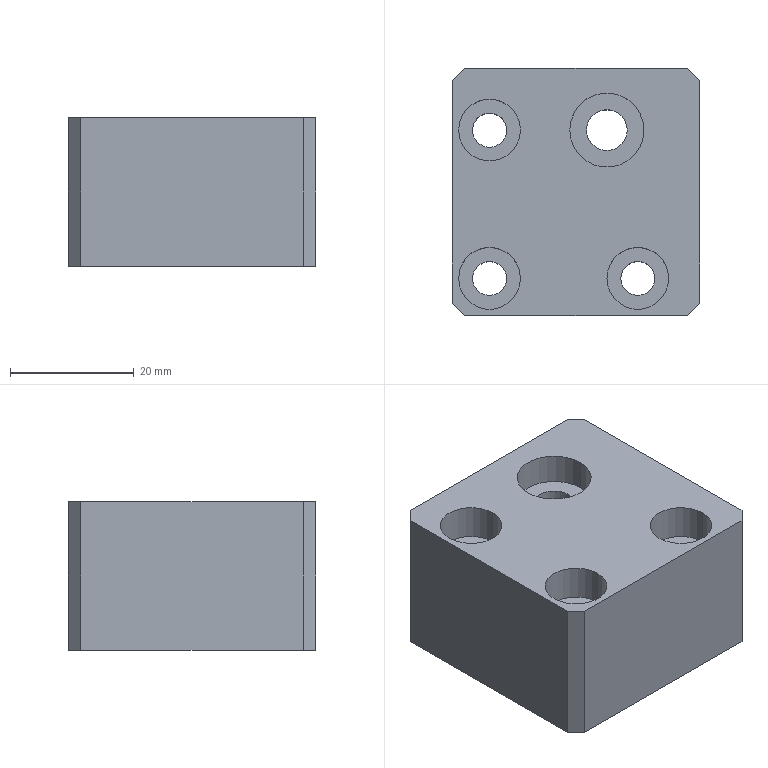Part | STEP file | 2008 Fixed block | 1 solid | 33 faces | box 40 x 40 x 24 mm | volume 33932 mm3 | cylinder 18 | plane 15 | commonest cylinder face diameters 5.5 x6 10 x6 6.6 x2 11 x2 12 x2